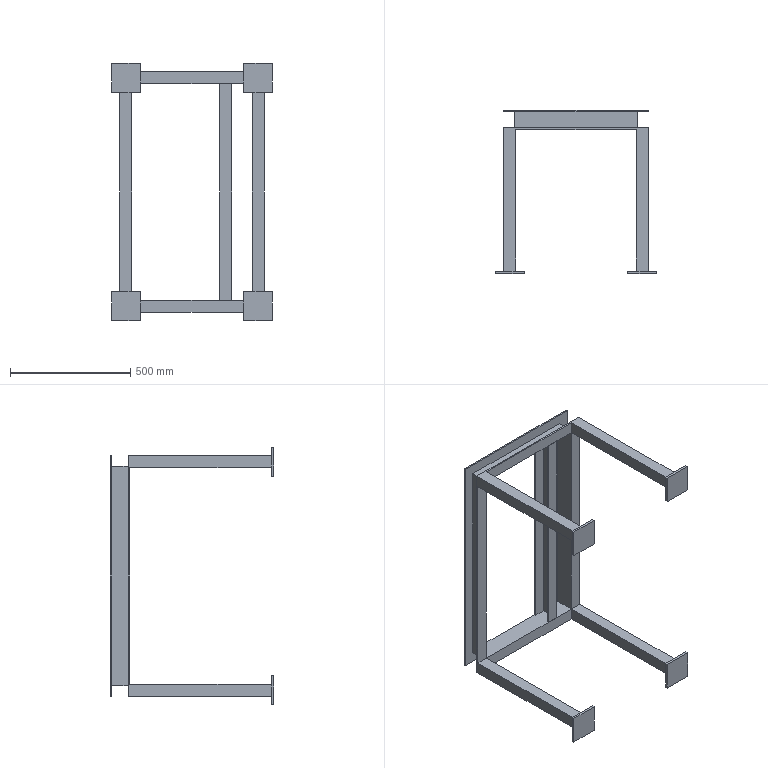Part | STEP file | Produce dryer line heating fan-SIROCCOFAN-3KW-001 | 2 solids | 65 faces | box 670 x 680 x 1070 mm | volume 10335392 mm3 | plane 65